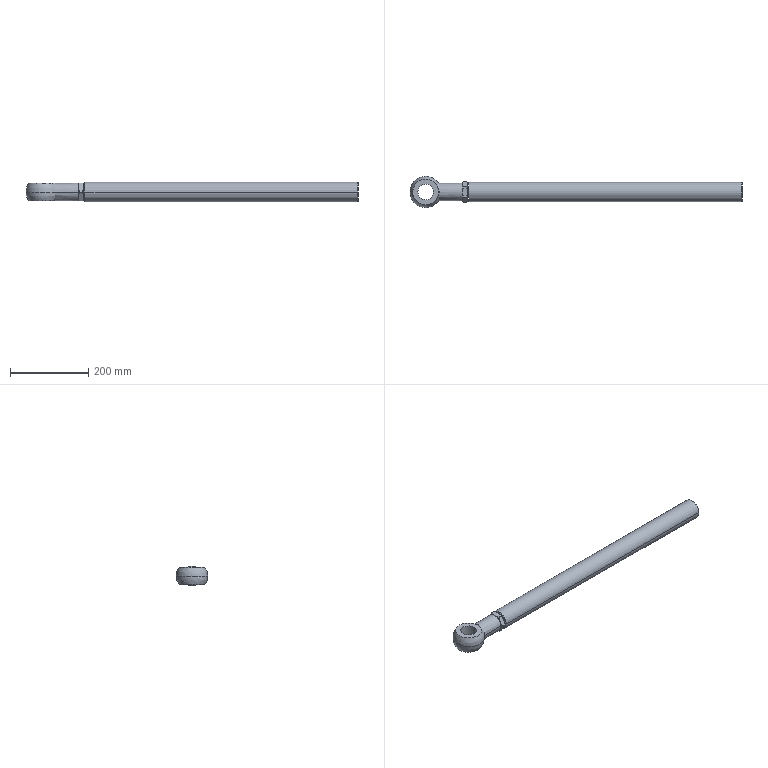Part | SolidWorks | features BaseBody 3 | 3 solids | 67 faces | box 850 x 80 x 50 mm | volume 1664669 mm3 | cone 28 | plane 27 | cylinder 10 | spline 2 | commonest cylinder face diameters 30 x6 40 x2 50 x2